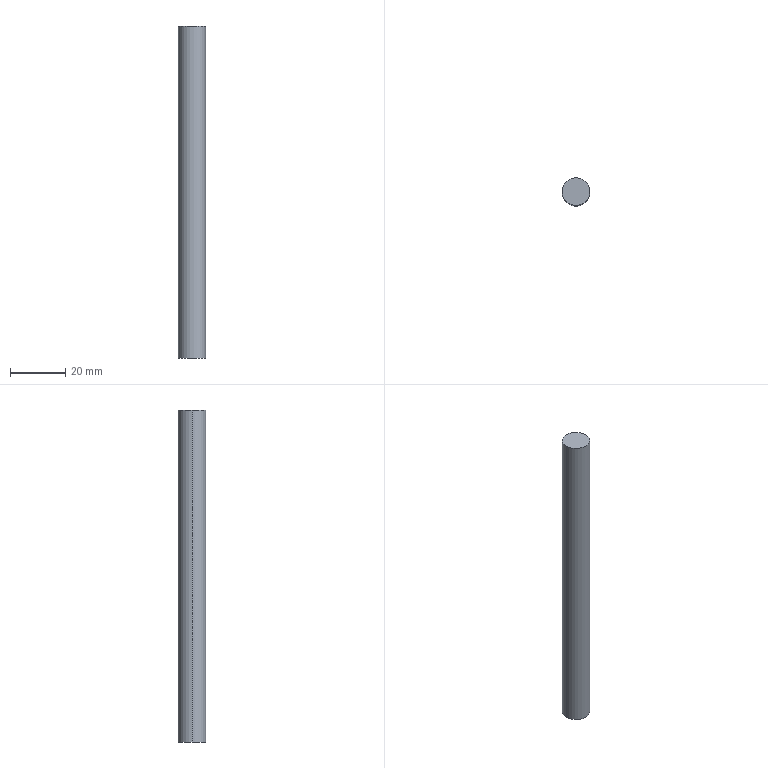Part | SolidWorks | 1 solid | 4 faces | box 10 x 10 x 120 mm | volume 9425 mm3 | plane 2 | cylinder 2 | commonest cylinder face diameters 10 x2
STEP:
#1=CARTESIAN_POINT('',(567.108,0.,50.));
#2=VERTEX_POINT('',#1);
#3=CARTESIAN_POINT('',(577.108,0.,50.));
#4=VERTEX_POINT('',#3);
#5=CARTESIAN_POINT('',(572.108,0.,50.));
#6=DIRECTION('',(0.,0.,1.));
#7=DIRECTION('',(-1.,0.,0.));
#8=AXIS2_PLACEMENT_3D('',#5,#6,#7);
#9=CIRCLE('',#8,5.);
#10=EDGE_CURVE('',#2,#4,#9,.T.);
#11=ORIENTED_EDGE('',*,*,#10,.F.);
#12=CARTESIAN_POINT('',(572.108,0.,50.));
#13=DIRECTION('',(0.,0.,1.));
#14=DIRECTION('',(1.,0.,0.));
#15=AXIS2_PLACEMENT_3D('',#12,#13,#14);
#16=CIRCLE('',#15,5.);
#17=EDGE_CURVE('',#4,#2,#16,.T.);
#18=ORIENTED_EDGE('',*,*,#17,.F.);
#19=EDGE_LOOP('',(#11,#18));
#20=FACE_OUTER_BOUND('',#19,.T.);
#21=CARTESIAN_POINT('',(572.108,0.,50.));
#22=DIRECTION('',(0.,0.,1.));
#23=DIRECTION('',(1.,0.,0.));
#24=AXIS2_PLACEMENT_3D('',#21,#22,#23);
#25=PLANE('',#24);
#26=ADVANCED_FACE('',(#20),#25,.F.);
#27=ORIENTED_EDGE('',*,*,#17,.T.);
#28=CARTESIAN_POINT('',(567.108,0.,170.));
#29=VERTEX_POINT('',#28);
#30=CARTESIAN_POINT('',(567.108,0.,50.));
#31=DIRECTION('',(0.,0.,1.));
#32=VECTOR('',#31,1000.);
#33=LINE('',#30,#32);
#34=EDGE_CURVE('',#2,#29,#33,.T.);
#35=ORIENTED_EDGE('',*,*,#34,.T.);
#36=CARTESIAN_POINT('',(577.108,0.,170.));
#37=VERTEX_POINT('',#36);
#38=CARTESIAN_POINT('',(572.108,0.,170.));
#39=DIRECTION('',(0.,0.,-1.));
#40=DIRECTION('',(-1.,0.,0.));
#41=AXIS2_PLACEMENT_3D('',#38,#39,#40);
#42=CIRCLE('',#41,5.);
#43=EDGE_CURVE('',#29,#37,#42,.T.);
#44=ORIENTED_EDGE('',*,*,#43,.T.);
#45=CARTESIAN_POINT('',(577.108,0.,50.));
#46=DIRECTION('',(0.,0.,1.));
#47=VECTOR('',#46,1000.);
#48=LINE('',#45,#47);
#49=EDGE_CURVE('',#4,#37,#48,.T.);
#50=ORIENTED_EDGE('',*,*,#49,.F.);
#51=EDGE_LOOP('',(#27,#35,#44,#50));
#52=FACE_OUTER_BOUND('',#51,.T.);
#53=CARTESIAN_POINT('',(572.108,0.,170.));
#54=DIRECTION('',(0.,0.,-1.));
#55=DIRECTION('',(-1.,0.,0.));
#56=AXIS2_PLACEMENT_3D('',#53,#54,#55);
#57=CYLINDRICAL_SURFACE('',#56,5.);
#58=ADVANCED_FACE('',(#52),#57,.T.);
#59=ORIENTED_EDGE('',*,*,#34,.F.);
#60=ORIENTED_EDGE('',*,*,#10,.T.);
#61=ORIENTED_EDGE('',*,*,#49,.T.);
#62=CARTESIAN_POINT('',(572.108,0.,170.));
#63=DIRECTION('',(0.,0.,-1.));
#64=DIRECTION('',(1.,0.,0.));
#65=AXIS2_PLACEMENT_3D('',#62,#63,#64);
#66=CIRCLE('',#65,5.);
#67=EDGE_CURVE('',#37,#29,#66,.T.);
#68=ORIENTED_EDGE('',*,*,#67,.T.);
#69=EDGE_LOOP('',(#59,#60,#61,#68));
#70=FACE_OUTER_BOUND('',#69,.T.);
#71=CARTESIAN_POINT('',(572.108,0.,170.));
#72=DIRECTION('',(0.,0.,-1.));
#73=DIRECTION('',(-1.,0.,0.));
#74=AXIS2_PLACEMENT_3D('',#71,#72,#73);
#75=CYLINDRICAL_SURFACE('',#74,5.);
#76=ADVANCED_FACE('',(#70),#75,.T.);
#77=ORIENTED_EDGE('',*,*,#43,.F.);
#78=ORIENTED_EDGE('',*,*,#67,.F.);
#79=EDGE_LOOP('',(#77,#78));
#80=FACE_OUTER_BOUND('',#79,.T.);
#81=CARTESIAN_POINT('',(572.108,0.,170.));
#82=DIRECTION('',(0.,0.,1.));
#83=DIRECTION('',(1.,0.,0.));
#84=AXIS2_PLACEMENT_3D('',#81,#82,#83);
#85=PLANE('',#84);
#86=ADVANCED_FACE('',(#80),#85,.T.);
#87=CLOSED_SHELL('',(#26,#58,#76,#86));
#88=MANIFOLD_SOLID_BREP('',#87);
#89=CARTESIAN_POINT('',(0.,0.,0.));
#90=DIRECTION('',(0.,0.,1.));
#91=DIRECTION('',(1.,0.,0.));
#92=AXIS2_PLACEMENT_3D('',#89,#90,#91);
#93=(LENGTH_UNIT()NAMED_UNIT(*)SI_UNIT(.MILLI.,.METRE.));
#94=UNCERTAINTY_MEASURE_WITH_UNIT(LENGTH_MEASURE(0.00001),#93,'','');
#95=(NAMED_UNIT(*)PLANE_ANGLE_UNIT()SI_UNIT($,.RADIAN.));
#96=(NAMED_UNIT(*)SI_UNIT($,.STERADIAN.)SOLID_ANGLE_UNIT());
#97=(GEOMETRIC_REPRESENTATION_CONTEXT(3)GLOBAL_UNCERTAINTY_ASSIGNED_CONTEXT((#94))GLOBAL_UNIT_ASSIGNED_CONTEXT((#93,#95,#96))REPRESENTATION_CONTEXT('',''));
#98=ADVANCED_BREP_SHAPE_REPRESENTATION('',(#88,#92),#97);